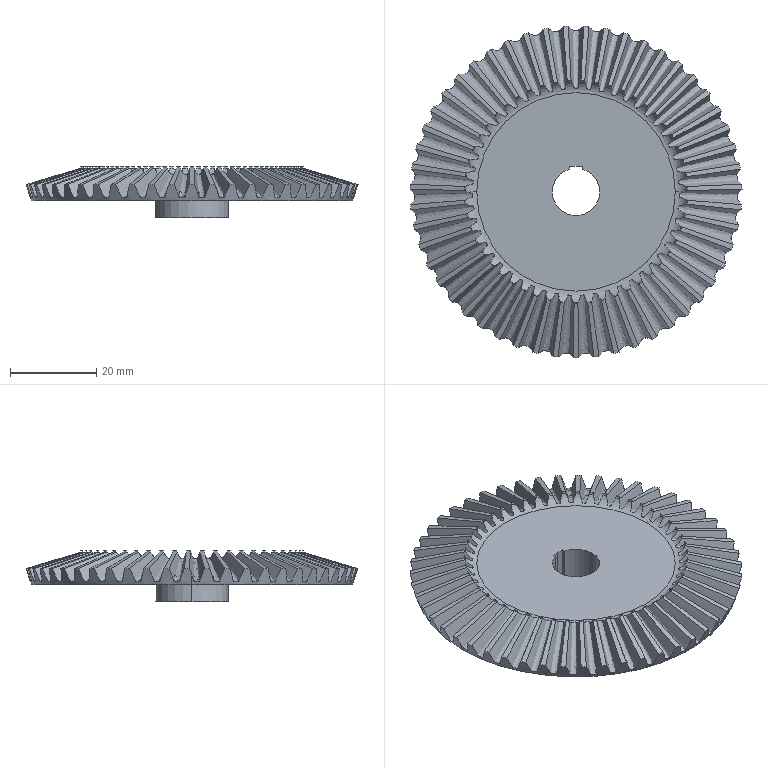Part | SolidWorks | features RefAxis 2, Revolution 2, BlendCut 1, CirPattern 1, ICE 1 | 1 solid | 271 faces | box 77.052 x 77.02 x 12.051 mm | volume 23159 mm3 | plane 108 | cone 104 | spline 51 | cylinder 6 | torus 2 | commonest cylinder face diameters 11 x3 17 x2 12 x1